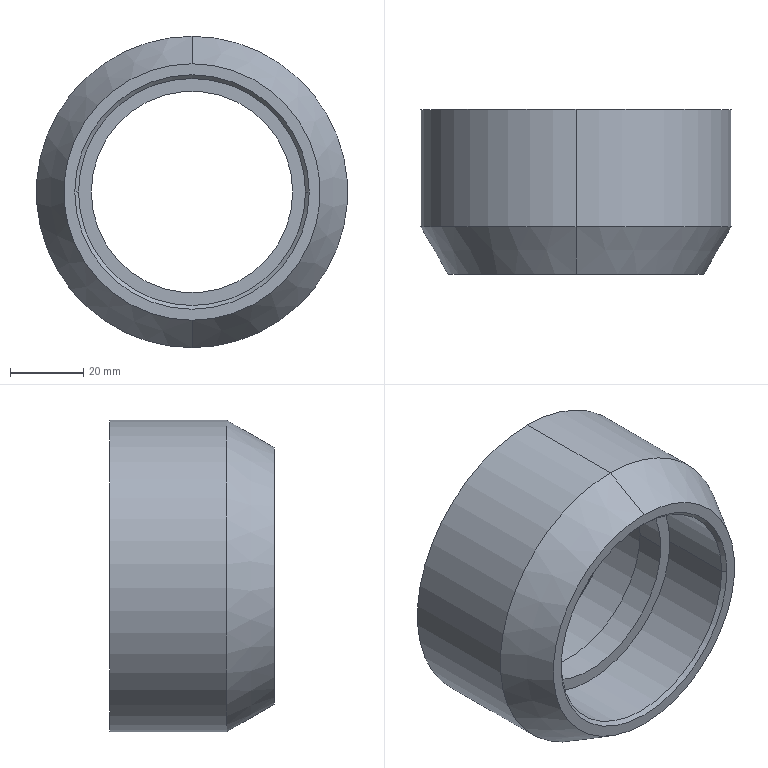Part | STEP file | 0229_216_Holder | 1 solid | 18 faces | box 85 x 45 x 85 mm | volume 112200 mm3 | cylinder 8 | cone 6 | plane 4 | commonest cylinder face diameters 62 x4 55 x2 85 x2
STEP:
#1=CARTESIAN_POINT('',(0.,0.,0.));
#2=DIRECTION('',(0.,0.,1.));
#3=DIRECTION('',(1.,0.,0.));
#4=AXIS2_PLACEMENT_3D('',#1,#2,#3);
#5=CARTESIAN_POINT('',(-31.,15.,0.));
#6=VERTEX_POINT('',#5);
#7=CARTESIAN_POINT('',(-32.,16.,0.));
#8=VERTEX_POINT('',#7);
#9=CARTESIAN_POINT('',(-31.,15.,0.));
#10=DIRECTION('',(-0.7071,0.7071,0.));
#11=VECTOR('',#10,1.);
#12=LINE('',#9,#11);
#13=CARTESIAN_POINT('',(0.,15.,0.));
#14=DIRECTION('',(0.,1.,0.));
#15=DIRECTION('',(-1.,0.,0.));
#16=AXIS2_PLACEMENT_3D('',#13,#14,#15);
#17=CONICAL_SURFACE('',#16,31.,0.7854);
#18=CARTESIAN_POINT('',(6.283,0.));
#19=DIRECTION('',(0.,1.));
#20=VECTOR('',#19,1.);
#21=LINE('',#18,#20);
#22=(GEOMETRIC_REPRESENTATION_CONTEXT(2)PARAMETRIC_REPRESENTATION_CONTEXT()REPRESENTATION_CONTEXT('',''));
#23=DEFINITIONAL_REPRESENTATION('',(#21),#22);
#24=PCURVE('',#17,#23);
#25=CARTESIAN_POINT('',(0.,15.,0.));
#26=DIRECTION('',(0.,1.,0.));
#27=DIRECTION('',(-1.,0.,0.));
#28=AXIS2_PLACEMENT_3D('',#25,#26,#27);
#29=CONICAL_SURFACE('',#28,31.,0.7854);
#30=CARTESIAN_POINT('',(0.,0.));
#31=DIRECTION('',(0.,1.));
#32=VECTOR('',#31,1.);
#33=LINE('',#30,#32);
#34=(GEOMETRIC_REPRESENTATION_CONTEXT(2)PARAMETRIC_REPRESENTATION_CONTEXT()REPRESENTATION_CONTEXT('',''));
#35=DEFINITIONAL_REPRESENTATION('',(#33),#34);
#36=PCURVE('',#29,#35);
#37=SURFACE_CURVE('',#12,(#24,#36),.PCURVE_S1.);
#38=EDGE_CURVE('',#6,#8,#37,.T.);
#39=ORIENTED_EDGE('',*,*,#38,.T.);
#40=CARTESIAN_POINT('',(32.,16.,0.));
#41=VERTEX_POINT('',#40);
#42=CARTESIAN_POINT('',(0.,16.,0.));
#43=DIRECTION('',(0.,-1.,0.));
#44=DIRECTION('',(0.,0.,-1.));
#45=AXIS2_PLACEMENT_3D('',#42,#43,#44);
#46=CIRCLE('',#45,32.);
#47=CARTESIAN_POINT('',(10.996,1.));
#48=DIRECTION('',(-1.,0.));
#49=VECTOR('',#48,1.);
#50=LINE('',#47,#49);
#51=(GEOMETRIC_REPRESENTATION_CONTEXT(2)PARAMETRIC_REPRESENTATION_CONTEXT()REPRESENTATION_CONTEXT('',''));
#52=DEFINITIONAL_REPRESENTATION('',(#50),#51);
#53=PCURVE('',#17,#52);
#54=CARTESIAN_POINT('',(0.,16.,0.));
#55=DIRECTION('',(0.,-1.,0.));
#56=DIRECTION('',(0.,0.,-1.));
#57=AXIS2_PLACEMENT_3D('',#54,#55,#56);
#58=PLANE('',#57);
#59=CARTESIAN_POINT('',(0.,0.));
#60=DIRECTION('',(1.,0.));
#61=AXIS2_PLACEMENT_2D('',#59,#60);
#62=CIRCLE('',#61,32.);
#63=(GEOMETRIC_REPRESENTATION_CONTEXT(2)PARAMETRIC_REPRESENTATION_CONTEXT()REPRESENTATION_CONTEXT('',''));
#64=DEFINITIONAL_REPRESENTATION('',(#62),#63);
#65=PCURVE('',#58,#64);
#66=SURFACE_CURVE('',#46,(#53,#65),.PCURVE_S1.);
#67=EDGE_CURVE('',#8,#41,#66,.T.);
#68=ORIENTED_EDGE('',*,*,#67,.T.);
#69=CARTESIAN_POINT('',(31.,15.,0.));
#70=VERTEX_POINT('',#69);
#71=CARTESIAN_POINT('',(31.,15.,0.));
#72=DIRECTION('',(0.7071,0.7071,0.));
#73=VECTOR('',#72,1.);
#74=LINE('',#71,#73);
#75=CARTESIAN_POINT('',(3.142,0.));
#76=DIRECTION('',(0.,1.));
#77=VECTOR('',#76,1.);
#78=LINE('',#75,#77);
#79=(GEOMETRIC_REPRESENTATION_CONTEXT(2)PARAMETRIC_REPRESENTATION_CONTEXT()REPRESENTATION_CONTEXT('',''));
#80=DEFINITIONAL_REPRESENTATION('',(#78),#79);
#81=PCURVE('',#17,#80);
#82=CARTESIAN_POINT('',(3.142,0.));
#83=DIRECTION('',(0.,1.));
#84=VECTOR('',#83,1.);
#85=LINE('',#82,#84);
#86=(GEOMETRIC_REPRESENTATION_CONTEXT(2)PARAMETRIC_REPRESENTATION_CONTEXT()REPRESENTATION_CONTEXT('',''));
#87=DEFINITIONAL_REPRESENTATION('',(#85),#86);
#88=PCURVE('',#29,#87);
#89=SURFACE_CURVE('',#74,(#81,#88),.PCURVE_S1.);
#90=EDGE_CURVE('',#70,#41,#89,.T.);
#91=ORIENTED_EDGE('',*,*,#90,.F.);
#92=CARTESIAN_POINT('',(0.,15.,0.));
#93=DIRECTION('',(0.,1.,0.));
#94=DIRECTION('',(1.,0.,0.));
#95=AXIS2_PLACEMENT_3D('',#92,#93,#94);
#96=CIRCLE('',#95,31.);
#97=CARTESIAN_POINT('',(3.142,0.));
#98=DIRECTION('',(1.,0.));
#99=VECTOR('',#98,1.);
#100=LINE('',#97,#99);
#101=(GEOMETRIC_REPRESENTATION_CONTEXT(2)PARAMETRIC_REPRESENTATION_CONTEXT()REPRESENTATION_CONTEXT('',''));
#102=DEFINITIONAL_REPRESENTATION('',(#100),#101);
#103=PCURVE('',#17,#102);
#104=CARTESIAN_POINT('',(0.,23.347,0.));
#105=DIRECTION('',(0.,1.,0.));
#106=DIRECTION('',(-1.,0.,0.));
#107=AXIS2_PLACEMENT_3D('',#104,#105,#106);
#108=CYLINDRICAL_SURFACE('',#107,31.);
#109=CARTESIAN_POINT('',(3.142,-8.347));
#110=DIRECTION('',(1.,0.));
#111=VECTOR('',#110,1.);
#112=LINE('',#109,#111);
#113=(GEOMETRIC_REPRESENTATION_CONTEXT(2)PARAMETRIC_REPRESENTATION_CONTEXT()REPRESENTATION_CONTEXT('',''));
#114=DEFINITIONAL_REPRESENTATION('',(#112),#113);
#115=PCURVE('',#108,#114);
#116=SURFACE_CURVE('',#96,(#103,#115),.PCURVE_S1.);
#117=EDGE_CURVE('',#70,#6,#116,.T.);
#118=ORIENTED_EDGE('',*,*,#117,.T.);
#119=EDGE_LOOP('',(#39,#68,#91,#118));
#120=FACE_BOUND('',#119,.F.);
#121=ADVANCED_FACE('',(#120),#17,.F.);
#122=CARTESIAN_POINT('',(31.,-28.,0.));
#123=VERTEX_POINT('',#122);
#124=CARTESIAN_POINT('',(32.,-29.,0.));
#125=VERTEX_POINT('',#124);
#126=CARTESIAN_POINT('',(32.,-29.,0.));
#127=DIRECTION('',(0.7071,-0.7071,0.));
#128=VECTOR('',#127,1.);
#129=LINE('',#126,#128);
#130=CARTESIAN_POINT('',(0.,-29.,0.));
#131=DIRECTION('',(0.,-1.,0.));
#132=DIRECTION('',(1.,0.,0.));
#133=AXIS2_PLACEMENT_3D('',#130,#131,#132);
#134=CONICAL_SURFACE('',#133,32.,0.7854);
#135=CARTESIAN_POINT('',(6.283,0.));
#136=DIRECTION('',(0.,1.));
#137=VECTOR('',#136,1.);
#138=LINE('',#135,#137);
#139=(GEOMETRIC_REPRESENTATION_CONTEXT(2)PARAMETRIC_REPRESENTATION_CONTEXT()REPRESENTATION_CONTEXT('',''));
#140=DEFINITIONAL_REPRESENTATION('',(#138),#139);
#141=PCURVE('',#134,#140);
#142=CARTESIAN_POINT('',(0.,-29.,0.));
#143=DIRECTION('',(0.,-1.,0.));
#144=DIRECTION('',(1.,0.,0.));
#145=AXIS2_PLACEMENT_3D('',#142,#143,#144);
#146=CONICAL_SURFACE('',#145,32.,0.7854);
#147=CARTESIAN_POINT('',(0.,0.));
#148=DIRECTION('',(0.,1.));
#149=VECTOR('',#148,1.);
#150=LINE('',#147,#149);
#151=(GEOMETRIC_REPRESENTATION_CONTEXT(2)PARAMETRIC_REPRESENTATION_CONTEXT()REPRESENTATION_CONTEXT('',''));
#152=DEFINITIONAL_REPRESENTATION('',(#150),#151);
#153=PCURVE('',#146,#152);
#154=SURFACE_CURVE('',#129,(#141,#153),.PCURVE_S1.);
#155=EDGE_CURVE('',#123,#125,#154,.T.);
#156=ORIENTED_EDGE('',*,*,#155,.T.);
#157=CARTESIAN_POINT('',(-32.,-29.,0.));
#158=VERTEX_POINT('',#157);
#159=CARTESIAN_POINT('',(0.,-29.,0.));
#160=DIRECTION('',(0.,1.,0.));
#161=DIRECTION('',(0.,0.,1.));
#162=AXIS2_PLACEMENT_3D('',#159,#160,#161);
#163=CIRCLE('',#162,32.);
#164=CARTESIAN_POINT('',(7.854,0.));
#165=DIRECTION('',(-1.,0.));
#166=VECTOR('',#165,1.);
#167=LINE('',#164,#166);
#168=(GEOMETRIC_REPRESENTATION_CONTEXT(2)PARAMETRIC_REPRESENTATION_CONTEXT()REPRESENTATION_CONTEXT('',''));
#169=DEFINITIONAL_REPRESENTATION('',(#167),#168);
#170=PCURVE('',#134,#169);
#171=CARTESIAN_POINT('',(0.,-29.,0.));
#172=DIRECTION('',(0.,1.,0.));
#173=DIRECTION('',(0.,0.,1.));
#174=AXIS2_PLACEMENT_3D('',#171,#172,#173);
#175=PLANE('',#174);
#176=CARTESIAN_POINT('',(0.,0.));
#177=DIRECTION('',(1.,0.));
#178=AXIS2_PLACEMENT_2D('',#176,#177);
#179=CIRCLE('',#178,32.);
#180=(GEOMETRIC_REPRESENTATION_CONTEXT(2)PARAMETRIC_REPRESENTATION_CONTEXT()REPRESENTATION_CONTEXT('',''));
#181=DEFINITIONAL_REPRESENTATION('',(#179),#180);
#182=PCURVE('',#175,#181);
#183=SURFACE_CURVE('',#163,(#170,#182),.PCURVE_S1.);
#184=EDGE_CURVE('',#125,#158,#183,.T.);
#185=ORIENTED_EDGE('',*,*,#184,.T.);
#186=CARTESIAN_POINT('',(-31.,-28.,0.));
#187=VERTEX_POINT('',#186);
#188=CARTESIAN_POINT('',(-32.,-29.,0.));
#189=DIRECTION('',(-0.7071,-0.7071,0.));
#190=VECTOR('',#189,1.);
#191=LINE('',#188,#190);
#192=CARTESIAN_POINT('',(3.142,0.));
#193=DIRECTION('',(0.,1.));
#194=VECTOR('',#193,1.);
#195=LINE('',#192,#194);
#196=(GEOMETRIC_REPRESENTATION_CONTEXT(2)PARAMETRIC_REPRESENTATION_CONTEXT()REPRESENTATION_CONTEXT('',''));
#197=DEFINITIONAL_REPRESENTATION('',(#195),#196);
#198=PCURVE('',#134,#197);
#199=CARTESIAN_POINT('',(3.142,0.));
#200=DIRECTION('',(0.,1.));
#201=VECTOR('',#200,1.);
#202=LINE('',#199,#201);
#203=(GEOMETRIC_REPRESENTATION_CONTEXT(2)PARAMETRIC_REPRESENTATION_CONTEXT()REPRESENTATION_CONTEXT('',''));
#204=DEFINITIONAL_REPRESENTATION('',(#202),#203);
#205=PCURVE('',#146,#204);
#206=SURFACE_CURVE('',#191,(#198,#205),.PCURVE_S1.);
#207=EDGE_CURVE('',#187,#158,#206,.T.);
#208=ORIENTED_EDGE('',*,*,#207,.F.);
#209=CARTESIAN_POINT('',(0.,-28.,0.));
#210=DIRECTION('',(0.,-1.,0.));
#211=DIRECTION('',(-1.,0.,0.));
#212=AXIS2_PLACEMENT_3D('',#209,#210,#211);
#213=CIRCLE('',#212,31.);
#214=CARTESIAN_POINT('',(3.142,-1.));
#215=DIRECTION('',(1.,0.));
#216=VECTOR('',#215,1.);
#217=LINE('',#214,#216);
#218=(GEOMETRIC_REPRESENTATION_CONTEXT(2)PARAMETRIC_REPRESENTATION_CONTEXT()REPRESENTATION_CONTEXT('',''));
#219=DEFINITIONAL_REPRESENTATION('',(#217),#218);
#220=PCURVE('',#134,#219);
#221=CARTESIAN_POINT('',(0.,23.347,0.));
#222=DIRECTION('',(0.,1.,0.));
#223=DIRECTION('',(-1.,0.,0.));
#224=AXIS2_PLACEMENT_3D('',#221,#222,#223);
#225=CYLINDRICAL_SURFACE('',#224,31.);
#226=CARTESIAN_POINT('',(6.283,-51.347));
#227=DIRECTION('',(-1.,0.));
#228=VECTOR('',#227,1.);
#229=LINE('',#226,#228);
#230=(GEOMETRIC_REPRESENTATION_CONTEXT(2)PARAMETRIC_REPRESENTATION_CONTEXT()REPRESENTATION_CONTEXT('',''));
#231=DEFINITIONAL_REPRESENTATION('',(#229),#230);
#232=PCURVE('',#225,#231);
#233=SURFACE_CURVE('',#213,(#220,#232),.PCURVE_S1.);
#234=EDGE_CURVE('',#187,#123,#233,.T.);
#235=ORIENTED_EDGE('',*,*,#234,.T.);
#236=EDGE_LOOP('',(#156,#185,#208,#235));
#237=FACE_BOUND('',#236,.F.);
#238=ADVANCED_FACE('',(#237),#134,.F.);
#239=CARTESIAN_POINT('',(0.,-29.,-35.));
#240=VERTEX_POINT('',#239);
#241=CARTESIAN_POINT('',(0.,-29.,35.));
#242=VERTEX_POINT('',#241);
#243=CARTESIAN_POINT('',(0.,-29.,0.));
#244=DIRECTION('',(0.,-1.,0.));
#245=DIRECTION('',(0.,0.,1.));
#246=AXIS2_PLACEMENT_3D('',#243,#244,#245);
#247=CIRCLE('',#246,35.);
#248=CARTESIAN_POINT('',(0.,-29.,0.));
#249=DIRECTION('',(0.,1.,0.));
#250=DIRECTION('',(0.,0.,1.));
#251=AXIS2_PLACEMENT_3D('',#248,#249,#250);
#252=CONICAL_SURFACE('',#251,35.,0.5236);
#253=CARTESIAN_POINT('',(6.283,0.));
#254=DIRECTION('',(-1.,0.));
#255=VECTOR('',#254,1.);
#256=LINE('',#253,#255);
#257=(GEOMETRIC_REPRESENTATION_CONTEXT(2)PARAMETRIC_REPRESENTATION_CONTEXT()REPRESENTATION_CONTEXT('',''));
#258=DEFINITIONAL_REPRESENTATION('',(#256),#257);
#259=PCURVE('',#252,#258);
#260=CARTESIAN_POINT('',(35.,0.));
#261=CARTESIAN_POINT('',(35.,-60.622));
#262=CARTESIAN_POINT('',(-17.5,-30.311));
#263=CARTESIAN_POINT('',(-70.,0.));
#264=CARTESIAN_POINT('',(-17.5,30.311));
#265=CARTESIAN_POINT('',(35.,60.622));
#266=CARTESIAN_POINT('',(35.,0.));
#267=(BOUNDED_CURVE()B_SPLINE_CURVE(2,(#260,#261,#262,#263,#264,#265,#266),.UNSPECIFIED.,.T.,.F.)B_SPLINE_CURVE_WITH_KNOTS((1,2,2,2,2,1),(-2.094,0.,2.094,4.189,6.283,8.378),.UNSPECIFIED.)CURVE()GEOMETRIC_REPRESENTATION_ITEM()RATIONAL_B_SPLINE_CURVE((1.,0.5,1.,0.5,1.,0.5,1.))REPRESENTATION_ITEM(''));
#268=(GEOMETRIC_REPRESENTATION_CONTEXT(2)PARAMETRIC_REPRESENTATION_CONTEXT()REPRESENTATION_CONTEXT('',''));
#269=DEFINITIONAL_REPRESENTATION('',(#267),#268);
#270=PCURVE('',#175,#269);
#271=SURFACE_CURVE('',#247,(#259,#270),.PCURVE_S1.);
#272=EDGE_CURVE('',#240,#242,#271,.T.);
#273=ORIENTED_EDGE('',*,*,#272,.F.);
#274=CARTESIAN_POINT('',(0.,-16.01,-42.5));
#275=VERTEX_POINT('',#274);
#276=CARTESIAN_POINT('',(0.,-29.,-35.));
#277=DIRECTION('',(0.,0.866,-0.5));
#278=VECTOR('',#277,1.);
#279=LINE('',#276,#278);
#280=CARTESIAN_POINT('',(3.142,0.));
#281=DIRECTION('',(0.,1.));
#282=VECTOR('',#281,1.);
#283=LINE('',#280,#282);
#284=(GEOMETRIC_REPRESENTATION_CONTEXT(2)PARAMETRIC_REPRESENTATION_CONTEXT()REPRESENTATION_CONTEXT('',''));
#285=DEFINITIONAL_REPRESENTATION('',(#283),#284);
#286=PCURVE('',#252,#285);
#287=CARTESIAN_POINT('',(0.,-29.,0.));
#288=DIRECTION('',(0.,1.,0.));
#289=DIRECTION('',(0.,0.,1.));
#290=AXIS2_PLACEMENT_3D('',#287,#288,#289);
#291=CONICAL_SURFACE('',#290,35.,0.5236);
#292=CARTESIAN_POINT('',(3.142,0.));
#293=DIRECTION('',(0.,1.));
#294=VECTOR('',#293,1.);
#295=LINE('',#292,#294);
#296=(GEOMETRIC_REPRESENTATION_CONTEXT(2)PARAMETRIC_REPRESENTATION_CONTEXT()REPRESENTATION_CONTEXT('',''));
#297=DEFINITIONAL_REPRESENTATION('',(#295),#296);
#298=PCURVE('',#291,#297);
#299=SURFACE_CURVE('',#279,(#286,#298),.PCURVE_S1.);
#300=EDGE_CURVE('',#240,#275,#299,.T.);
#301=ORIENTED_EDGE('',*,*,#300,.T.);
#302=CARTESIAN_POINT('',(0.,-16.01,42.5));
#303=VERTEX_POINT('',#302);
#304=CARTESIAN_POINT('',(0.,-16.01,0.));
#305=DIRECTION('',(0.,1.,0.));
#306=DIRECTION('',(0.,0.,1.));
#307=AXIS2_PLACEMENT_3D('',#304,#305,#306);
#308=CIRCLE('',#307,42.5);
#309=CARTESIAN_POINT('',(0.,12.99));
#310=DIRECTION('',(1.,0.));
#311=VECTOR('',#310,1.);
#312=LINE('',#309,#311);
#313=(GEOMETRIC_REPRESENTATION_CONTEXT(2)PARAMETRIC_REPRESENTATION_CONTEXT()REPRESENTATION_CONTEXT('',''));
#314=DEFINITIONAL_REPRESENTATION('',(#312),#313);
#315=PCURVE('',#252,#314);
#316=CARTESIAN_POINT('',(0.,-41.143,0.));
#317=DIRECTION('',(0.,-1.,0.));
#318=DIRECTION('',(0.,0.,-1.));
#319=AXIS2_PLACEMENT_3D('',#316,#317,#318);
#320=CYLINDRICAL_SURFACE('',#319,42.5);
#321=CARTESIAN_POINT('',(3.142,-25.133));
#322=DIRECTION('',(-1.,0.));
#323=VECTOR('',#322,1.);
#324=LINE('',#321,#323);
#325=(GEOMETRIC_REPRESENTATION_CONTEXT(2)PARAMETRIC_REPRESENTATION_CONTEXT()REPRESENTATION_CONTEXT('',''));
#326=DEFINITIONAL_REPRESENTATION('',(#324),#325);
#327=PCURVE('',#320,#326);
#328=SURFACE_CURVE('',#308,(#315,#327),.PCURVE_S1.);
#329=EDGE_CURVE('',#303,#275,#328,.T.);
#330=ORIENTED_EDGE('',*,*,#329,.F.);
#331=CARTESIAN_POINT('',(0.,-29.,35.));
#332=DIRECTION('',(0.,0.866,0.5));
#333=VECTOR('',#332,1.);
#334=LINE('',#331,#333);
#335=CARTESIAN_POINT('',(0.,0.));
#336=DIRECTION('',(0.,1.));
#337=VECTOR('',#336,1.);
#338=LINE('',#335,#337);
#339=(GEOMETRIC_REPRESENTATION_CONTEXT(2)PARAMETRIC_REPRESENTATION_CONTEXT()REPRESENTATION_CONTEXT('',''));
#340=DEFINITIONAL_REPRESENTATION('',(#338),#339);
#341=PCURVE('',#252,#340);
#342=CARTESIAN_POINT('',(6.283,0.));
#343=DIRECTION('',(0.,1.));
#344=VECTOR('',#343,1.);
#345=LINE('',#342,#344);
#346=(GEOMETRIC_REPRESENTATION_CONTEXT(2)PARAMETRIC_REPRESENTATION_CONTEXT()REPRESENTATION_CONTEXT('',''));
#347=DEFINITIONAL_REPRESENTATION('',(#345),#346);
#348=PCURVE('',#291,#347);
#349=SURFACE_CURVE('',#334,(#341,#348),.PCURVE_S1.);
#350=EDGE_CURVE('',#242,#303,#349,.T.);
#351=ORIENTED_EDGE('',*,*,#350,.F.);
#352=EDGE_LOOP('',(#273,#301,#330,#351));
#353=FACE_BOUND('',#352,.T.);
#354=ADVANCED_FACE('',(#353),#252,.T.);
#355=CARTESIAN_POINT('',(-31.,-8.,0.));
#356=VERTEX_POINT('',#355);
#357=CARTESIAN_POINT('',(-31.,23.347,0.));
#358=DIRECTION('',(0.,1.,0.));
#359=VECTOR('',#358,1.);
#360=LINE('',#357,#359);
#361=CARTESIAN_POINT('',(6.283,0.));
#362=DIRECTION('',(0.,1.));
#363=VECTOR('',#362,1.);
#364=LINE('',#361,#363);
#365=(GEOMETRIC_REPRESENTATION_CONTEXT(2)PARAMETRIC_REPRESENTATION_CONTEXT()REPRESENTATION_CONTEXT('',''));
#366=DEFINITIONAL_REPRESENTATION('',(#364),#365);
#367=PCURVE('',#225,#366);
#368=CARTESIAN_POINT('',(0.,23.347,0.));
#369=DIRECTION('',(0.,1.,0.));
#370=DIRECTION('',(-1.,0.,0.));
#371=AXIS2_PLACEMENT_3D('',#368,#369,#370);
#372=CYLINDRICAL_SURFACE('',#371,31.);
#373=CARTESIAN_POINT('',(0.,0.));
#374=DIRECTION('',(0.,1.));
#375=VECTOR('',#374,1.);
#376=LINE('',#373,#375);
#377=(GEOMETRIC_REPRESENTATION_CONTEXT(2)PARAMETRIC_REPRESENTATION_CONTEXT()REPRESENTATION_CONTEXT('',''));
#378=DEFINITIONAL_REPRESENTATION('',(#376),#377);
#379=PCURVE('',#372,#378);
#380=SURFACE_CURVE('',#360,(#367,#379),.PCURVE_S1.);
#381=EDGE_CURVE('',#187,#356,#380,.T.);
#382=ORIENTED_EDGE('',*,*,#381,.T.);
#383=CARTESIAN_POINT('',(31.,-8.,0.));
#384=VERTEX_POINT('',#383);
#385=CARTESIAN_POINT('',(0.,-8.,0.));
#386=DIRECTION('',(0.,1.,0.));
#387=DIRECTION('',(-1.,0.,0.));
#388=AXIS2_PLACEMENT_3D('',#385,#386,#387);
#389=CIRCLE('',#388,31.);
#390=CARTESIAN_POINT('',(0.,-31.347));
#391=DIRECTION('',(1.,0.));
#392=VECTOR('',#391,1.);
#393=LINE('',#390,#392);
#394=(GEOMETRIC_REPRESENTATION_CONTEXT(2)PARAMETRIC_REPRESENTATION_CONTEXT()REPRESENTATION_CONTEXT('',''));
#395=DEFINITIONAL_REPRESENTATION('',(#393),#394);
#396=PCURVE('',#225,#395);
#397=CARTESIAN_POINT('',(-27.5,-8.,0.));
#398=DIRECTION('',(0.,1.,0.));
#399=DIRECTION('',(-1.,0.,0.));
#400=AXIS2_PLACEMENT_3D('',#397,#398,#399);
#401=PLANE('',#400);
#402=CARTESIAN_POINT('',(-27.5,0.));
#403=DIRECTION('',(1.,0.));
#404=AXIS2_PLACEMENT_2D('',#402,#403);
#405=CIRCLE('',#404,31.);
#406=(GEOMETRIC_REPRESENTATION_CONTEXT(2)PARAMETRIC_REPRESENTATION_CONTEXT()REPRESENTATION_CONTEXT('',''));
#407=DEFINITIONAL_REPRESENTATION('',(#405),#406);
#408=PCURVE('',#401,#407);
#409=SURFACE_CURVE('',#389,(#396,#408),.PCURVE_S1.);
#410=EDGE_CURVE('',#384,#356,#409,.T.);
#411=ORIENTED_EDGE('',*,*,#410,.F.);
#412=CARTESIAN_POINT('',(31.,23.347,0.));
#413=DIRECTION('',(0.,1.,0.));
#414=VECTOR('',#413,1.);
#415=LINE('',#412,#414);
#416=CARTESIAN_POINT('',(3.142,0.));
#417=DIRECTION('',(0.,1.));
#418=VECTOR('',#417,1.);
#419=LINE('',#416,#418);
#420=(GEOMETRIC_REPRESENTATION_CONTEXT(2)PARAMETRIC_REPRESENTATION_CONTEXT()REPRESENTATION_CONTEXT('',''));
#421=DEFINITIONAL_REPRESENTATION('',(#419),#420);
#422=PCURVE('',#225,#421);
#423=CARTESIAN_POINT('',(3.142,0.));
#424=DIRECTION('',(0.,1.));
#425=VECTOR('',#424,1.);
#426=LINE('',#423,#425);
#427=(GEOMETRIC_REPRESENTATION_CONTEXT(2)PARAMETRIC_REPRESENTATION_CONTEXT()REPRESENTATION_CONTEXT('',''));
#428=DEFINITIONAL_REPRESENTATION('',(#426),#427);
#429=PCURVE('',#372,#428);
#430=SURFACE_CURVE('',#415,(#422,#429),.PCURVE_S1.);
#431=EDGE_CURVE('',#123,#384,#430,.T.);
#432=ORIENTED_EDGE('',*,*,#431,.F.);
#433=ORIENTED_EDGE('',*,*,#234,.F.);
#434=EDGE_LOOP('',(#382,#411,#432,#433));
#435=FACE_BOUND('',#434,.F.);
#436=ADVANCED_FACE('',(#435),#225,.F.);
#437=CARTESIAN_POINT('',(-27.5,-8.,0.));
#438=VERTEX_POINT('',#437);
#439=CARTESIAN_POINT('',(-27.5,0.,0.));
#440=VERTEX_POINT('',#439);
#441=CARTESIAN_POINT('',(-27.5,23.347,0.));
#442=DIRECTION('',(0.,1.,0.));
#443=VECTOR('',#442,1.);
#444=LINE('',#441,#443);
#445=CARTESIAN_POINT('',(0.,23.347,0.));
#446=DIRECTION('',(0.,1.,0.));
#447=DIRECTION('',(-1.,0.,0.));
#448=AXIS2_PLACEMENT_3D('',#445,#446,#447);
#449=CYLINDRICAL_SURFACE('',#448,27.5);
#450=CARTESIAN_POINT('',(6.283,0.));
#451=DIRECTION('',(0.,1.));
#452=VECTOR('',#451,1.);
#453=LINE('',#450,#452);
#454=(GEOMETRIC_REPRESENTATION_CONTEXT(2)PARAMETRIC_REPRESENTATION_CONTEXT()REPRESENTATION_CONTEXT('',''));
#455=DEFINITIONAL_REPRESENTATION('',(#453),#454);
#456=PCURVE('',#449,#455);
#457=CARTESIAN_POINT('',(0.,23.347,0.));
#458=DIRECTION('',(0.,1.,0.));
#459=DIRECTION('',(-1.,0.,0.));
#460=AXIS2_PLACEMENT_3D('',#457,#458,#459);
#461=CYLINDRICAL_SURFACE('',#460,27.5);
#462=CARTESIAN_POINT('',(0.,0.));
#463=DIRECTION('',(0.,1.));
#464=VECTOR('',#463,1.);
#465=LINE('',#462,#464);
#466=(GEOMETRIC_REPRESENTATION_CONTEXT(2)PARAMETRIC_REPRESENTATION_CONTEXT()REPRESENTATION_CONTEXT('',''));
#467=DEFINITIONAL_REPRESENTATION('',(#465),#466);
#468=PCURVE('',#461,#467);
#469=SURFACE_CURVE('',#444,(#456,#468),.PCURVE_S1.);
#470=EDGE_CURVE('',#438,#440,#469,.T.);
#471=ORIENTED_EDGE('',*,*,#470,.T.);
#472=CARTESIAN_POINT('',(27.5,0.,0.));
#473=VERTEX_POINT('',#472);
#474=CARTESIAN_POINT('',(0.,0.,0.));
#475=DIRECTION('',(0.,1.,0.));
#476=DIRECTION('',(-1.,0.,0.));
#477=AXIS2_PLACEMENT_3D('',#474,#475,#476);
#478=CIRCLE('',#477,27.5);
#479=CARTESIAN_POINT('',(0.,-23.347));
#480=DIRECTION('',(1.,0.));
#481=VECTOR('',#480,1.);
#482=LINE('',#479,#481);
#483=(GEOMETRIC_REPRESENTATION_CONTEXT(2)PARAMETRIC_REPRESENTATION_CONTEXT()REPRESENTATION_CONTEXT('',''));
#484=DEFINITIONAL_REPRESENTATION('',(#482),#483);
#485=PCURVE('',#449,#484);
#486=CARTESIAN_POINT('',(-31.,0.,0.));
#487=DIRECTION('',(0.,-1.,0.));
#488=DIRECTION('',(1.,0.,0.));
#489=AXIS2_PLACEMENT_3D('',#486,#487,#488);
#490=PLANE('',#489);
#491=CARTESIAN_POINT('',(3.5,0.));
#492=CARTESIAN_POINT('',(3.5,47.631));
#493=CARTESIAN_POINT('',(44.75,23.816));
#494=CARTESIAN_POINT('',(86.,0.));
#495=CARTESIAN_POINT('',(44.75,-23.816));
#496=CARTESIAN_POINT('',(3.5,-47.631));
#497=CARTESIAN_POINT('',(3.5,0.));
#498=(BOUNDED_CURVE()B_SPLINE_CURVE(2,(#491,#492,#493,#494,#495,#496,#497),.UNSPECIFIED.,.T.,.F.)B_SPLINE_CURVE_WITH_KNOTS((1,2,2,2,2,1),(-2.094,0.,2.094,4.189,6.283,8.378),.UNSPECIFIED.)CURVE()GEOMETRIC_REPRESENTATION_ITEM()RATIONAL_B_SPLINE_CURVE((1.,0.5,1.,0.5,1.,0.5,1.))REPRESENTATION_ITEM(''));
#499=(GEOMETRIC_REPRESENTATION_CONTEXT(2)PARAMETRIC_REPRESENTATION_CONTEXT()REPRESENTATION_CONTEXT('',''));
#500=DEFINITIONAL_REPRESENTATION('',(#498),#499);
#501=PCURVE('',#490,#500);
#502=SURFACE_CURVE('',#478,(#485,#501),.PCURVE_S1.);
#503=EDGE_CURVE('',#473,#440,#502,.T.);
#504=ORIENTED_EDGE('',*,*,#503,.F.);
#505=CARTESIAN_POINT('',(27.5,-8.,0.));
#506=VERTEX_POINT('',#505);
#507=CARTESIAN_POINT('',(27.5,23.347,0.));
#508=DIRECTION('',(0.,1.,0.));
#509=VECTOR('',#508,1.);
#510=LINE('',#507,#509);
#511=CARTESIAN_POINT('',(3.142,0.));
#512=DIRECTION('',(0.,1.));
#513=VECTOR('',#512,1.);
#514=LINE('',#511,#513);
#515=(GEOMETRIC_REPRESENTATION_CONTEXT(2)PARAMETRIC_REPRESENTATION_CONTEXT()REPRESENTATION_CONTEXT('',''));
#516=DEFINITIONAL_REPRESENTATION('',(#514),#515);
#517=PCURVE('',#449,#516);
#518=CARTESIAN_POINT('',(3.142,0.));
#519=DIRECTION('',(0.,1.));
#520=VECTOR('',#519,1.);
#521=LINE('',#518,#520);
#522=(GEOMETRIC_REPRESENTATION_CONTEXT(2)PARAMETRIC_REPRESENTATION_CONTEXT()REPRESENTATION_CONTEXT('',''));
#523=DEFINITIONAL_REPRESENTATION('',(#521),#522);
#524=PCURVE('',#461,#523);
#525=SURFACE_CURVE('',#510,(#517,#524),.PCURVE_S1.);
#526=EDGE_CURVE('',#506,#473,#525,.T.);
#527=ORIENTED_EDGE('',*,*,#526,.F.);
#528=CARTESIAN_POINT('',(0.,-8.,0.));
#529=DIRECTION('',(0.,1.,0.));
#530=DIRECTION('',(-1.,0.,0.));
#531=AXIS2_PLACEMENT_3D('',#528,#529,#530);
#532=CIRCLE('',#531,27.5);
#533=CARTESIAN_POINT('',(0.,-31.347));
#534=DIRECTION('',(1.,0.));
#535=VECTOR('',#534,1.);
#536=LINE('',#533,#535);
#537=(GEOMETRIC_REPRESENTATION_CONTEXT(2)PARAMETRIC_REPRESENTATION_CONTEXT()REPRESENTATION_CONTEXT('',''));
#538=DEFINITIONAL_REPRESENTATION('',(#536),#537);
#539=PCURVE('',#449,#538);
#540=CARTESIAN_POINT('',(-27.5,0.));
#541=DIRECTION('',(1.,0.));
#542=AXIS2_PLACEMENT_2D('',#540,#541);
#543=CIRCLE('',#542,27.5);
#544=(GEOMETRIC_REPRESENTATION_CONTEXT(2)PARAMETRIC_REPRESENTATION_CONTEXT()REPRESENTATION_CONTEXT('',''));
#545=DEFINITIONAL_REPRESENTATION('',(#543),#544);
#546=PCURVE('',#401,#545);
#547=SURFACE_CURVE('',#532,(#539,#546),.PCURVE_S1.);
#548=EDGE_CURVE('',#506,#438,#547,.T.);
#549=ORIENTED_EDGE('',*,*,#548,.T.);
#550=EDGE_LOOP('',(#471,#504,#527,#549));
#551=FACE_BOUND('',#550,.F.);
#552=ADVANCED_FACE('',(#551),#449,.F.);
#553=CARTESIAN_POINT('',(-31.,0.,0.));
#554=VERTEX_POINT('',#553);
#555=CARTESIAN_POINT('',(-31.,23.347,0.));
#556=DIRECTION('',(0.,1.,0.));
#557=VECTOR('',#556,1.);
#558=LINE('',#555,#557);
#559=CARTESIAN_POINT('',(6.283,0.));
#560=DIRECTION('',(0.,1.));
#561=VECTOR('',#560,1.);
#562=LINE('',#559,#561);
#563=(GEOMETRIC_REPRESENTATION_CONTEXT(2)PARAMETRIC_REPRESENTATION_CONTEXT()REPRESENTATION_CONTEXT('',''));
#564=DEFINITIONAL_REPRESENTATION('',(#562),#563);
#565=PCURVE('',#108,#564);
#566=CARTESIAN_POINT('',(0.,23.347,0.));
#567=DIRECTION('',(0.,1.,0.));
#568=DIRECTION('',(-1.,0.,0.));
#569=AXIS2_PLACEMENT_3D('',#566,#567,#568);
#570=CYLINDRICAL_SURFACE('',#569,31.);
#571=CARTESIAN_POINT('',(0.,0.));
#572=DIRECTION('',(0.,1.));
#573=VECTOR('',#572,1.);
#574=LINE('',#571,#573);
#575=(GEOMETRIC_REPRESENTATION_CONTEXT(2)PARAMETRIC_REPRESENTATION_CONTEXT()REPRESENTATION_CONTEXT('',''));
#576=DEFINITIONAL_REPRESENTATION('',(#574),#575);
#577=PCURVE('',#570,#576);
#578=SURFACE_CURVE('',#558,(#565,#577),.PCURVE_S1.);
#579=EDGE_CURVE('',#554,#6,#578,.T.);
#580=ORIENTED_EDGE('',*,*,#579,.T.);
#581=ORIENTED_EDGE('',*,*,#117,.F.);
#582=CARTESIAN_POINT('',(31.,0.,0.));
#583=VERTEX_POINT('',#582);
#584=CARTESIAN_POINT('',(31.,23.347,0.));
#585=DIRECTION('',(0.,1.,0.));
#586=VECTOR('',#585,1.);
#587=LINE('',#584,#586);
#588=CARTESIAN_POINT('',(3.142,0.));
#589=DIRECTION('',(0.,1.));
#590=VECTOR('',#589,1.);
#591=LINE('',#588,#590);
#592=(GEOMETRIC_REPRESENTATION_CONTEXT(2)PARAMETRIC_REPRESENTATION_CONTEXT()REPRESENTATION_CONTEXT('',''));
#593=DEFINITIONAL_REPRESENTATION('',(#591),#592);
#594=PCURVE('',#108,#593);
#595=CARTESIAN_POINT('',(3.142,0.));
#596=DIRECTION('',(0.,1.));
#597=VECTOR('',#596,1.);
#598=LINE('',#595,#597);
#599=(GEOMETRIC_REPRESENTATION_CONTEXT(2)PARAMETRIC_REPRESENTATION_CONTEXT()REPRESENTATION_CONTEXT('',''));
#600=DEFINITIONAL_REPRESENTATION('',(#598),#599);
#601=PCURVE('',#570,#600);
#602=SURFACE_CURVE('',#587,(#594,#601),.PCURVE_S1.);
#603=EDGE_CURVE('',#583,#70,#602,.T.);
#604=ORIENTED_EDGE('',*,*,#603,.F.);
#605=CARTESIAN_POINT('',(0.,0.,0.));
#606=DIRECTION('',(0.,1.,0.));
#607=DIRECTION('',(-1.,0.,0.));
#608=AXIS2_PLACEMENT_3D('',#605,#606,#607);
#609=CIRCLE('',#608,31.);
#610=CARTESIAN_POINT('',(0.,-23.347));
#611=DIRECTION('',(1.,0.));
#612=VECTOR('',#611,1.);
#613=LINE('',#610,#612);
#614=(GEOMETRIC_REPRESENTATION_CONTEXT(2)PARAMETRIC_REPRESENTATION_CONTEXT()REPRESENTATION_CONTEXT('',''));
#615=DEFINITIONAL_REPRESENTATION('',(#613),#614);
#616=PCURVE('',#108,#615);
#617=CARTESIAN_POINT('',(0.,0.));
#618=CARTESIAN_POINT('',(0.,53.694));
#619=CARTESIAN_POINT('',(46.5,26.847));
#620=CARTESIAN_POINT('',(93.,0.));
#621=CARTESIAN_POINT('',(46.5,-26.847));
#622=CARTESIAN_POINT('',(0.,-53.694));
#623=CARTESIAN_POINT('',(0.,0.));
#624=(BOUNDED_CURVE()B_SPLINE_CURVE(2,(#617,#618,#619,#620,#621,#622,#623),.UNSPECIFIED.,.T.,.F.)B_SPLINE_CURVE_WITH_KNOTS((1,2,2,2,2,1),(-2.094,0.,2.094,4.189,6.283,8.378),.UNSPECIFIED.)CURVE()GEOMETRIC_REPRESENTATION_ITEM()RATIONAL_B_SPLINE_CURVE((1.,0.5,1.,0.5,1.,0.5,1.))REPRESENTATION_ITEM(''));
#625=(GEOMETRIC_REPRESENTATION_CONTEXT(2)PARAMETRIC_REPRESENTATION_CONTEXT()REPRESENTATION_CONTEXT('',''));
#626=DEFINITIONAL_REPRESENTATION('',(#624),#625);
#627=PCURVE('',#490,#626);
#628=SURFACE_CURVE('',#609,(#616,#627),.PCURVE_S1.);
#629=EDGE_CURVE('',#583,#554,#628,.T.);
#630=ORIENTED_EDGE('',*,*,#629,.T.);
#631=EDGE_LOOP('',(#580,#581,#604,#630));
#632=FACE_BOUND('',#631,.F.);
#633=ADVANCED_FACE('',(#632),#108,.F.);
#634=CARTESIAN_POINT('',(0.,16.,-42.5));
#635=VERTEX_POINT('',#634);
#636=CARTESIAN_POINT('',(0.,16.,42.5));
#637=VERTEX_POINT('',#636);
#638=CARTESIAN_POINT('',(0.,16.,0.));
#639=DIRECTION('',(0.,-1.,0.));
#640=DIRECTION('',(0.,0.,-1.));
#641=AXIS2_PLACEMENT_3D('',#638,#639,#640);
#642=CIRCLE('',#641,42.5);
#643=CARTESIAN_POINT('',(0.,-57.143));
#644=DIRECTION('',(1.,0.));
#645=VECTOR('',#644,1.);
#646=LINE('',#643,#645);
#647=(GEOMETRIC_REPRESENTATION_CONTEXT(2)PARAMETRIC_REPRESENTATION_CONTEXT()REPRESENTATION_CONTEXT('',''));
#648=DEFINITIONAL_REPRESENTATION('',(#646),#647);
#649=PCURVE('',#320,#648);
#650=CARTESIAN_POINT('',(0.,0.));
#651=DIRECTION('',(1.,0.));
#652=AXIS2_PLACEMENT_2D('',#650,#651);
#653=CIRCLE('',#652,42.5);
#654=(GEOMETRIC_REPRESENTATION_CONTEXT(2)PARAMETRIC_REPRESENTATION_CONTEXT()REPRESENTATION_CONTEXT('',''));
#655=DEFINITIONAL_REPRESENTATION('',(#653),#654);
#656=PCURVE('',#58,#655);
#657=SURFACE_CURVE('',#642,(#649,#656),.PCURVE_S1.);
#658=EDGE_CURVE('',#635,#637,#657,.T.);
#659=ORIENTED_EDGE('',*,*,#658,.T.);
#660=CARTESIAN_POINT('',(0.,-41.143,42.5));
#661=DIRECTION('',(0.,-1.,0.));
#662=VECTOR('',#661,1.);
#663=LINE('',#660,#662);
#664=CARTESIAN_POINT('',(3.142,0.));
#665=DIRECTION('',(0.,1.));
#666=VECTOR('',#665,1.);
#667=LINE('',#664,#666);
#668=(GEOMETRIC_REPRESENTATION_CONTEXT(2)PARAMETRIC_REPRESENTATION_CONTEXT()REPRESENTATION_CONTEXT('',''));
#669=DEFINITIONAL_REPRESENTATION('',(#667),#668);
#670=PCURVE('',#320,#669);
#671=CARTESIAN_POINT('',(0.,-41.143,0.));
#672=DIRECTION('',(0.,-1.,0.));
#673=DIRECTION('',(0.,0.,-1.));
#674=AXIS2_PLACEMENT_3D('',#671,#672,#673);
#675=CYLINDRICAL_SURFACE('',#674,42.5);
#676=CARTESIAN_POINT('',(3.142,0.));
#677=DIRECTION('',(0.,1.));
#678=VECTOR('',#677,1.);
#679=LINE('',#676,#678);
#680=(GEOMETRIC_REPRESENTATION_CONTEXT(2)PARAMETRIC_REPRESENTATION_CONTEXT()REPRESENTATION_CONTEXT('',''));
#681=DEFINITIONAL_REPRESENTATION('',(#679),#680);
#682=PCURVE('',#675,#681);
#683=SURFACE_CURVE('',#663,(#670,#682),.PCURVE_S1.);
#684=EDGE_CURVE('',#637,#303,#683,.T.);
#685=ORIENTED_EDGE('',*,*,#684,.T.);
#686=ORIENTED_EDGE('',*,*,#329,.T.);
#687=CARTESIAN_POINT('',(0.,-41.143,-42.5));
#688=DIRECTION('',(0.,-1.,0.));
#689=VECTOR('',#688,1.);
#690=LINE('',#687,#689);
#691=CARTESIAN_POINT('',(0.,0.));
#692=DIRECTION('',(0.,1.));
#693=VECTOR('',#692,1.);
#694=LINE('',#691,#693);
#695=(GEOMETRIC_REPRESENTATION_CONTEXT(2)PARAMETRIC_REPRESENTATION_CONTEXT()REPRESENTATION_CONTEXT('',''));
#696=DEFINITIONAL_REPRESENTATION('',(#694),#695);
#697=PCURVE('',#320,#696);
#698=CARTESIAN_POINT('',(6.283,0.));
#699=DIRECTION('',(0.,1.));
#700=VECTOR('',#699,1.);
#701=LINE('',#698,#700);
#702=(GEOMETRIC_REPRESENTATION_CONTEXT(2)PARAMETRIC_REPRESENTATION_CONTEXT()REPRESENTATION_CONTEXT('',''));
#703=DEFINITIONAL_REPRESENTATION('',(#701),#702);
#704=PCURVE('',#675,#703);
#705=SURFACE_CURVE('',#690,(#697,#704),.PCURVE_S1.);
#706=EDGE_CURVE('',#635,#275,#705,.T.);
#707=ORIENTED_EDGE('',*,*,#706,.F.);
#708=EDGE_LOOP('',(#659,#685,#686,#707));
#709=FACE_BOUND('',#708,.T.);
#710=ADVANCED_FACE('',(#709),#320,.T.);
#711=ORIENTED_EDGE('',*,*,#184,.T.);
#712=CARTESIAN_POINT('',(0.,-29.,0.));
#713=DIRECTION('',(0.,1.,0.));
#714=DIRECTION('',(0.,0.,1.));
#715=AXIS2_PLACEMENT_3D('',#712,#713,#714);
#716=CIRCLE('',#715,32.);
#717=CARTESIAN_POINT('',(0.,0.));
#718=DIRECTION('',(1.,0.));
#719=AXIS2_PLACEMENT_2D('',#717,#718);
#720=CIRCLE('',#719,32.);
#721=(GEOMETRIC_REPRESENTATION_CONTEXT(2)PARAMETRIC_REPRESENTATION_CONTEXT()REPRESENTATION_CONTEXT('',''));
#722=DEFINITIONAL_REPRESENTATION('',(#720),#721);
#723=PCURVE('',#175,#722);
#724=CARTESIAN_POINT('',(7.854,0.));
#725=DIRECTION('',(-1.,0.));
#726=VECTOR('',#725,1.);
#727=LINE('',#724,#726);
#728=(GEOMETRIC_REPRESENTATION_CONTEXT(2)PARAMETRIC_REPRESENTATION_CONTEXT()REPRESENTATION_CONTEXT('',''));
#729=DEFINITIONAL_REPRESENTATION('',(#727),#728);
#730=PCURVE('',#146,#729);
#731=SURFACE_CURVE('',#716,(#723,#730),.PCURVE_S1.);
#732=EDGE_CURVE('',#158,#125,#731,.T.);
#733=ORIENTED_EDGE('',*,*,#732,.T.);
#734=EDGE_LOOP('',(#711,#733));
#735=FACE_BOUND('',#734,.T.);
#736=CARTESIAN_POINT('',(0.,-29.,0.));
#737=DIRECTION('',(0.,-1.,0.));
#738=DIRECTION('',(0.,0.,1.));
#739=AXIS2_PLACEMENT_3D('',#736,#737,#738);
#740=CIRCLE('',#739,35.);
#741=CARTESIAN_POINT('',(35.,0.));
#742=CARTESIAN_POINT('',(35.,-60.622));
#743=CARTESIAN_POINT('',(-17.5,-30.311));
#744=CARTESIAN_POINT('',(-70.,0.));
#745=CARTESIAN_POINT('',(-17.5,30.311));
#746=CARTESIAN_POINT('',(35.,60.622));
#747=CARTESIAN_POINT('',(35.,0.));
#748=(BOUNDED_CURVE()B_SPLINE_CURVE(2,(#741,#742,#743,#744,#745,#746,#747),.UNSPECIFIED.,.T.,.F.)B_SPLINE_CURVE_WITH_KNOTS((1,2,2,2,2,1),(-2.094,0.,2.094,4.189,6.283,8.378),.UNSPECIFIED.)CURVE()GEOMETRIC_REPRESENTATION_ITEM()RATIONAL_B_SPLINE_CURVE((1.,0.5,1.,0.5,1.,0.5,1.))REPRESENTATION_ITEM(''));
#749=(GEOMETRIC_REPRESENTATION_CONTEXT(2)PARAMETRIC_REPRESENTATION_CONTEXT()REPRESENTATION_CONTEXT('',''));
#750=DEFINITIONAL_REPRESENTATION('',(#748),#749);
#751=PCURVE('',#175,#750);
#752=CARTESIAN_POINT('',(6.283,0.));
#753=DIRECTION('',(-1.,0.));
#754=VECTOR('',#753,1.);
#755=LINE('',#752,#754);
#756=(GEOMETRIC_REPRESENTATION_CONTEXT(2)PARAMETRIC_REPRESENTATION_CONTEXT()REPRESENTATION_CONTEXT('',''));
#757=DEFINITIONAL_REPRESENTATION('',(#755),#756);
#758=PCURVE('',#291,#757);
#759=SURFACE_CURVE('',#740,(#751,#758),.PCURVE_S1.);
#760=EDGE_CURVE('',#242,#240,#759,.T.);
#761=ORIENTED_EDGE('',*,*,#760,.T.);
#762=ORIENTED_EDGE('',*,*,#272,.T.);
#763=EDGE_LOOP('',(#761,#762));
#764=FACE_BOUND('',#763,.T.);
#765=ADVANCED_FACE('',(#735,#764),#175,.F.);
#766=ORIENTED_EDGE('',*,*,#684,.F.);
#767=CARTESIAN_POINT('',(0.,16.,0.));
#768=DIRECTION('',(0.,-1.,0.));
#769=DIRECTION('',(0.,0.,-1.));
#770=AXIS2_PLACEMENT_3D('',#767,#768,#769);
#771=CIRCLE('',#770,42.5);
#772=CARTESIAN_POINT('',(0.,-57.143));
#773=DIRECTION('',(1.,0.));
#774=VECTOR('',#773,1.);
#775=LINE('',#772,#774);
#776=(GEOMETRIC_REPRESENTATION_CONTEXT(2)PARAMETRIC_REPRESENTATION_CONTEXT()REPRESENTATION_CONTEXT('',''));
#777=DEFINITIONAL_REPRESENTATION('',(#775),#776);
#778=PCURVE('',#675,#777);
#779=CARTESIAN_POINT('',(0.,0.));
#780=DIRECTION('',(1.,0.));
#781=AXIS2_PLACEMENT_2D('',#779,#780);
#782=CIRCLE('',#781,42.5);
#783=(GEOMETRIC_REPRESENTATION_CONTEXT(2)PARAMETRIC_REPRESENTATION_CONTEXT()REPRESENTATION_CONTEXT('',''));
#784=DEFINITIONAL_REPRESENTATION('',(#782),#783);
#785=PCURVE('',#58,#784);
#786=SURFACE_CURVE('',#771,(#778,#785),.PCURVE_S1.);
#787=EDGE_CURVE('',#637,#635,#786,.T.);
#788=ORIENTED_EDGE('',*,*,#787,.T.);
#789=ORIENTED_EDGE('',*,*,#706,.T.);
#790=CARTESIAN_POINT('',(0.,-16.01,0.));
#791=DIRECTION('',(0.,1.,0.));
#792=DIRECTION('',(0.,0.,1.));
#793=AXIS2_PLACEMENT_3D('',#790,#791,#792);
#794=CIRCLE('',#793,42.5);
#795=CARTESIAN_POINT('',(9.425,-25.133));
#796=DIRECTION('',(-1.,0.));
#797=VECTOR('',#796,1.);
#798=LINE('',#795,#797);
#799=(GEOMETRIC_REPRESENTATION_CONTEXT(2)PARAMETRIC_REPRESENTATION_CONTEXT()REPRESENTATION_CONTEXT('',''));
#800=DEFINITIONAL_REPRESENTATION('',(#798),#799);
#801=PCURVE('',#675,#800);
#802=CARTESIAN_POINT('',(0.,12.99));
#803=DIRECTION('',(1.,0.));
#804=VECTOR('',#803,1.);
#805=LINE('',#802,#804);
#806=(GEOMETRIC_REPRESENTATION_CONTEXT(2)PARAMETRIC_REPRESENTATION_CONTEXT()REPRESENTATION_CONTEXT('',''));
#807=DEFINITIONAL_REPRESENTATION('',(#805),#806);
#808=PCURVE('',#291,#807);
#809=SURFACE_CURVE('',#794,(#801,#808),.PCURVE_S1.);
#810=EDGE_CURVE('',#275,#303,#809,.T.);
#811=ORIENTED_EDGE('',*,*,#810,.T.);
#812=EDGE_LOOP('',(#766,#788,#789,#811));
#813=FACE_BOUND('',#812,.T.);
#814=ADVANCED_FACE('',(#813),#675,.T.);
#815=ORIENTED_EDGE('',*,*,#67,.T.);
#816=CARTESIAN_POINT('',(0.,16.,0.));
#817=DIRECTION('',(0.,-1.,0.));
#818=DIRECTION('',(0.,0.,-1.));
#819=AXIS2_PLACEMENT_3D('',#816,#817,#818);
#820=CIRCLE('',#819,32.);
#821=CARTESIAN_POINT('',(0.,0.));
#822=DIRECTION('',(1.,0.));
#823=AXIS2_PLACEMENT_2D('',#821,#822);
#824=CIRCLE('',#823,32.);
#825=(GEOMETRIC_REPRESENTATION_CONTEXT(2)PARAMETRIC_REPRESENTATION_CONTEXT()REPRESENTATION_CONTEXT('',''));
#826=DEFINITIONAL_REPRESENTATION('',(#824),#825);
#827=PCURVE('',#58,#826);
#828=CARTESIAN_POINT('',(4.712,1.));
#829=DIRECTION('',(-1.,0.));
#830=VECTOR('',#829,1.);
#831=LINE('',#828,#830);
#832=(GEOMETRIC_REPRESENTATION_CONTEXT(2)PARAMETRIC_REPRESENTATION_CONTEXT()REPRESENTATION_CONTEXT('',''));
#833=DEFINITIONAL_REPRESENTATION('',(#831),#832);
#834=PCURVE('',#29,#833);
#835=SURFACE_CURVE('',#820,(#827,#834),.PCURVE_S1.);
#836=EDGE_CURVE('',#41,#8,#835,.T.);
#837=ORIENTED_EDGE('',*,*,#836,.T.);
#838=EDGE_LOOP('',(#815,#837));
#839=FACE_BOUND('',#838,.T.);
#840=ORIENTED_EDGE('',*,*,#658,.F.);
#841=ORIENTED_EDGE('',*,*,#787,.F.);
#842=EDGE_LOOP('',(#840,#841));
#843=FACE_BOUND('',#842,.T.);
#844=ADVANCED_FACE('',(#839,#843),#58,.F.);
#845=CARTESIAN_POINT('',(0.,15.,0.));
#846=DIRECTION('',(0.,1.,0.));
#847=DIRECTION('',(1.,0.,0.));
#848=AXIS2_PLACEMENT_3D('',#845,#846,#847);
#849=CIRCLE('',#848,31.);
#850=CARTESIAN_POINT('',(-3.142,-8.347));
#851=DIRECTION('',(1.,0.));
#852=VECTOR('',#851,1.);
#853=LINE('',#850,#852);
#854=(GEOMETRIC_REPRESENTATION_CONTEXT(2)PARAMETRIC_REPRESENTATION_CONTEXT()REPRESENTATION_CONTEXT('',''));
#855=DEFINITIONAL_REPRESENTATION('',(#853),#854);
#856=PCURVE('',#570,#855);
#857=CARTESIAN_POINT('',(-3.142,0.));
#858=DIRECTION('',(1.,0.));
#859=VECTOR('',#858,1.);
#860=LINE('',#857,#859);
#861=(GEOMETRIC_REPRESENTATION_CONTEXT(2)PARAMETRIC_REPRESENTATION_CONTEXT()REPRESENTATION_CONTEXT('',''));
#862=DEFINITIONAL_REPRESENTATION('',(#860),#861);
#863=PCURVE('',#29,#862);
#864=SURFACE_CURVE('',#849,(#856,#863),.PCURVE_S1.);
#865=EDGE_CURVE('',#6,#70,#864,.T.);
#866=ORIENTED_EDGE('',*,*,#865,.F.);
#867=ORIENTED_EDGE('',*,*,#579,.F.);
#868=CARTESIAN_POINT('',(0.,0.,0.));
#869=DIRECTION('',(0.,1.,0.));
#870=DIRECTION('',(-1.,0.,0.));
#871=AXIS2_PLACEMENT_3D('',#868,#869,#870);
#872=CIRCLE('',#871,31.);
#873=CARTESIAN_POINT('',(0.,-23.347));
#874=DIRECTION('',(1.,0.));
#875=VECTOR('',#874,1.);
#876=LINE('',#873,#875);
#877=(GEOMETRIC_REPRESENTATION_CONTEXT(2)PARAMETRIC_REPRESENTATION_CONTEXT()REPRESENTATION_CONTEXT('',''));
#878=DEFINITIONAL_REPRESENTATION('',(#876),#877);
#879=PCURVE('',#570,#878);
#880=CARTESIAN_POINT('',(0.,0.));
#881=CARTESIAN_POINT('',(0.,53.694));
#882=CARTESIAN_POINT('',(46.5,26.847));
#883=CARTESIAN_POINT('',(93.,0.));
#884=CARTESIAN_POINT('',(46.5,-26.847));
#885=CARTESIAN_POINT('',(0.,-53.694));
#886=CARTESIAN_POINT('',(0.,0.));
#887=(BOUNDED_CURVE()B_SPLINE_CURVE(2,(#880,#881,#882,#883,#884,#885,#886),.UNSPECIFIED.,.T.,.F.)B_SPLINE_CURVE_WITH_KNOTS((1,2,2,2,2,1),(-2.094,0.,2.094,4.189,6.283,8.378),.UNSPECIFIED.)CURVE()GEOMETRIC_REPRESENTATION_ITEM()RATIONAL_B_SPLINE_CURVE((1.,0.5,1.,0.5,1.,0.5,1.))REPRESENTATION_ITEM(''));
#888=(GEOMETRIC_REPRESENTATION_CONTEXT(2)PARAMETRIC_REPRESENTATION_CONTEXT()REPRESENTATION_CONTEXT('',''));
#889=DEFINITIONAL_REPRESENTATION('',(#887),#888);
#890=PCURVE('',#490,#889);
#891=SURFACE_CURVE('',#872,(#879,#890),.PCURVE_S1.);
#892=EDGE_CURVE('',#554,#583,#891,.T.);
#893=ORIENTED_EDGE('',*,*,#892,.T.);
#894=ORIENTED_EDGE('',*,*,#603,.T.);
#895=EDGE_LOOP('',(#866,#867,#893,#894));
#896=FACE_BOUND('',#895,.F.);
#897=ADVANCED_FACE('',(#896),#570,.F.);
#898=CARTESIAN_POINT('',(0.,0.,0.));
#899=DIRECTION('',(0.,1.,0.));
#900=DIRECTION('',(-1.,0.,0.));
#901=AXIS2_PLACEMENT_3D('',#898,#899,#900);
#902=CIRCLE('',#901,27.5);
#903=CARTESIAN_POINT('',(3.5,0.));
#904=CARTESIAN_POINT('',(3.5,47.631));
#905=CARTESIAN_POINT('',(44.75,23.816));
#906=CARTESIAN_POINT('',(86.,0.));
#907=CARTESIAN_POINT('',(44.75,-23.816));
#908=CARTESIAN_POINT('',(3.5,-47.631));
#909=CARTESIAN_POINT('',(3.5,0.));
#910=(BOUNDED_CURVE()B_SPLINE_CURVE(2,(#903,#904,#905,#906,#907,#908,#909),.UNSPECIFIED.,.T.,.F.)B_SPLINE_CURVE_WITH_KNOTS((1,2,2,2,2,1),(-2.094,0.,2.094,4.189,6.283,8.378),.UNSPECIFIED.)CURVE()GEOMETRIC_REPRESENTATION_ITEM()RATIONAL_B_SPLINE_CURVE((1.,0.5,1.,0.5,1.,0.5,1.))REPRESENTATION_ITEM(''));
#911=(GEOMETRIC_REPRESENTATION_CONTEXT(2)PARAMETRIC_REPRESENTATION_CONTEXT()REPRESENTATION_CONTEXT('',''));
#912=DEFINITIONAL_REPRESENTATION('',(#910),#911);
#913=PCURVE('',#490,#912);
#914=CARTESIAN_POINT('',(0.,-23.347));
#915=DIRECTION('',(1.,0.));
#916=VECTOR('',#915,1.);
#917=LINE('',#914,#916);
#918=(GEOMETRIC_REPRESENTATION_CONTEXT(2)PARAMETRIC_REPRESENTATION_CONTEXT()REPRESENTATION_CONTEXT('',''));
#919=DEFINITIONAL_REPRESENTATION('',(#917),#918);
#920=PCURVE('',#461,#919);
#921=SURFACE_CURVE('',#902,(#913,#920),.PCURVE_S1.);
#922=EDGE_CURVE('',#440,#473,#921,.T.);
#923=ORIENTED_EDGE('',*,*,#922,.F.);
#924=ORIENTED_EDGE('',*,*,#503,.F.);
#925=EDGE_LOOP('',(#923,#924));
#926=FACE_BOUND('',#925,.T.);
#927=ORIENTED_EDGE('',*,*,#892,.T.);
#928=ORIENTED_EDGE('',*,*,#629,.T.);
#929=EDGE_LOOP('',(#927,#928));
#930=FACE_BOUND('',#929,.T.);
#931=ADVANCED_FACE('',(#926,#930),#490,.F.);
#932=ORIENTED_EDGE('',*,*,#922,.F.);
#933=ORIENTED_EDGE('',*,*,#470,.F.);
#934=CARTESIAN_POINT('',(0.,-8.,0.));
#935=DIRECTION('',(0.,1.,0.));
#936=DIRECTION('',(-1.,0.,0.));
#937=AXIS2_PLACEMENT_3D('',#934,#935,#936);
#938=CIRCLE('',#937,27.5);
#939=CARTESIAN_POINT('',(0.,-31.347));
#940=DIRECTION('',(1.,0.));
#941=VECTOR('',#940,1.);
#942=LINE('',#939,#941);
#943=(GEOMETRIC_REPRESENTATION_CONTEXT(2)PARAMETRIC_REPRESENTATION_CONTEXT()REPRESENTATION_CONTEXT('',''));
#944=DEFINITIONAL_REPRESENTATION('',(#942),#943);
#945=PCURVE('',#461,#944);
#946=CARTESIAN_POINT('',(-27.5,0.));
#947=DIRECTION('',(1.,0.));
#948=AXIS2_PLACEMENT_2D('',#946,#947);
#949=CIRCLE('',#948,27.5);
#950=(GEOMETRIC_REPRESENTATION_CONTEXT(2)PARAMETRIC_REPRESENTATION_CONTEXT()REPRESENTATION_CONTEXT('',''));
#951=DEFINITIONAL_REPRESENTATION('',(#949),#950);
#952=PCURVE('',#401,#951);
#953=SURFACE_CURVE('',#938,(#945,#952),.PCURVE_S1.);
#954=EDGE_CURVE('',#438,#506,#953,.T.);
#955=ORIENTED_EDGE('',*,*,#954,.T.);
#956=ORIENTED_EDGE('',*,*,#526,.T.);
#957=EDGE_LOOP('',(#932,#933,#955,#956));
#958=FACE_BOUND('',#957,.F.);
#959=ADVANCED_FACE('',(#958),#461,.F.);
#960=CARTESIAN_POINT('',(0.,-8.,0.));
#961=DIRECTION('',(0.,1.,0.));
#962=DIRECTION('',(-1.,0.,0.));
#963=AXIS2_PLACEMENT_3D('',#960,#961,#962);
#964=CIRCLE('',#963,31.);
#965=CARTESIAN_POINT('',(-27.5,0.));
#966=DIRECTION('',(1.,0.));
#967=AXIS2_PLACEMENT_2D('',#965,#966);
#968=CIRCLE('',#967,31.);
#969=(GEOMETRIC_REPRESENTATION_CONTEXT(2)PARAMETRIC_REPRESENTATION_CONTEXT()REPRESENTATION_CONTEXT('',''));
#970=DEFINITIONAL_REPRESENTATION('',(#968),#969);
#971=PCURVE('',#401,#970);
#972=CARTESIAN_POINT('',(0.,-31.347));
#973=DIRECTION('',(1.,0.));
#974=VECTOR('',#973,1.);
#975=LINE('',#972,#974);
#976=(GEOMETRIC_REPRESENTATION_CONTEXT(2)PARAMETRIC_REPRESENTATION_CONTEXT()REPRESENTATION_CONTEXT('',''));
#977=DEFINITIONAL_REPRESENTATION('',(#975),#976);
#978=PCURVE('',#372,#977);
#979=SURFACE_CURVE('',#964,(#971,#978),.PCURVE_S1.);
#980=EDGE_CURVE('',#356,#384,#979,.T.);
#981=ORIENTED_EDGE('',*,*,#980,.F.);
#982=ORIENTED_EDGE('',*,*,#410,.F.);
#983=EDGE_LOOP('',(#981,#982));
#984=FACE_BOUND('',#983,.T.);
#985=ORIENTED_EDGE('',*,*,#954,.T.);
#986=ORIENTED_EDGE('',*,*,#548,.T.);
#987=EDGE_LOOP('',(#985,#986));
#988=FACE_BOUND('',#987,.T.);
#989=ADVANCED_FACE('',(#984,#988),#401,.F.);
#990=ORIENTED_EDGE('',*,*,#980,.F.);
#991=ORIENTED_EDGE('',*,*,#381,.F.);
#992=CARTESIAN_POINT('',(0.,-28.,0.));
#993=DIRECTION('',(0.,-1.,0.));
#994=DIRECTION('',(-1.,0.,0.));
#995=AXIS2_PLACEMENT_3D('',#992,#993,#994);
#996=CIRCLE('',#995,31.);
#997=CARTESIAN_POINT('',(6.283,-51.347));
#998=DIRECTION('',(-1.,0.));
#999=VECTOR('',#998,1.);
#1000=LINE('',#997,#999);
#1001=(GEOMETRIC_REPRESENTATION_CONTEXT(2)PARAMETRIC_REPRESENTATION_CONTEXT()REPRESENTATION_CONTEXT('',''));
#1002=DEFINITIONAL_REPRESENTATION('',(#1000),#1001);
#1003=PCURVE('',#372,#1002);
#1004=CARTESIAN_POINT('',(-3.142,-1.));
#1005=DIRECTION('',(1.,0.));
#1006=VECTOR('',#1005,1.);
#1007=LINE('',#1004,#1006);
#1008=(GEOMETRIC_REPRESENTATION_CONTEXT(2)PARAMETRIC_REPRESENTATION_CONTEXT()REPRESENTATION_CONTEXT('',''));
#1009=DEFINITIONAL_REPRESENTATION('',(#1007),#1008);
#1010=PCURVE('',#146,#1009);
#1011=SURFACE_CURVE('',#996,(#1003,#1010),.PCURVE_S1.);
#1012=EDGE_CURVE('',#123,#187,#1011,.T.);
#1013=ORIENTED_EDGE('',*,*,#1012,.F.);
#1014=ORIENTED_EDGE('',*,*,#431,.T.);
#1015=EDGE_LOOP('',(#990,#991,#1013,#1014));
#1016=FACE_BOUND('',#1015,.F.);
#1017=ADVANCED_FACE('',(#1016),#372,.F.);
#1018=ORIENTED_EDGE('',*,*,#300,.F.);
#1019=ORIENTED_EDGE('',*,*,#760,.F.);
#1020=ORIENTED_EDGE('',*,*,#350,.T.);
#1021=ORIENTED_EDGE('',*,*,#810,.F.);
#1022=EDGE_LOOP('',(#1018,#1019,#1020,#1021));
#1023=FACE_BOUND('',#1022,.T.);
#1024=ADVANCED_FACE('',(#1023),#291,.T.);
#1025=ORIENTED_EDGE('',*,*,#732,.T.);
#1026=ORIENTED_EDGE('',*,*,#155,.F.);
#1027=ORIENTED_EDGE('',*,*,#1012,.T.);
#1028=ORIENTED_EDGE('',*,*,#207,.T.);
#1029=EDGE_LOOP('',(#1025,#1026,#1027,#1028));
#1030=FACE_BOUND('',#1029,.F.);
#1031=ADVANCED_FACE('',(#1030),#146,.F.);
#1032=ORIENTED_EDGE('',*,*,#836,.T.);
#1033=ORIENTED_EDGE('',*,*,#38,.F.);
#1034=ORIENTED_EDGE('',*,*,#865,.T.);
#1035=ORIENTED_EDGE('',*,*,#90,.T.);
#1036=EDGE_LOOP('',(#1032,#1033,#1034,#1035));
#1037=FACE_BOUND('',#1036,.F.);
#1038=ADVANCED_FACE('',(#1037),#29,.F.);
#1039=CLOSED_SHELL('',(#121,#238,#354,#436,#552,#633,#710,#765,#814,#844,#897,#931,#959,#989,#1017,#1024,#1031,#1038));
#1040=MANIFOLD_SOLID_BREP('',#1039);
#1041=(LENGTH_UNIT()NAMED_UNIT(*)SI_UNIT(.MILLI.,.METRE.));
#1042=UNCERTAINTY_MEASURE_WITH_UNIT(LENGTH_MEASURE(0.0000001),#1041,'','');
#1043=(NAMED_UNIT(*)PLANE_ANGLE_UNIT()SI_UNIT($,.RADIAN.));
#1044=(NAMED_UNIT(*)SI_UNIT($,.STERADIAN.)SOLID_ANGLE_UNIT());
#1045=(GEOMETRIC_REPRESENTATION_CONTEXT(3)GLOBAL_UNCERTAINTY_ASSIGNED_CONTEXT((#1042))GLOBAL_UNIT_ASSIGNED_CONTEXT((#1041,#1043,#1044))REPRESENTATION_CONTEXT('',''));
#1046=ADVANCED_BREP_SHAPE_REPRESENTATION('',(#4,#1040),#1045);